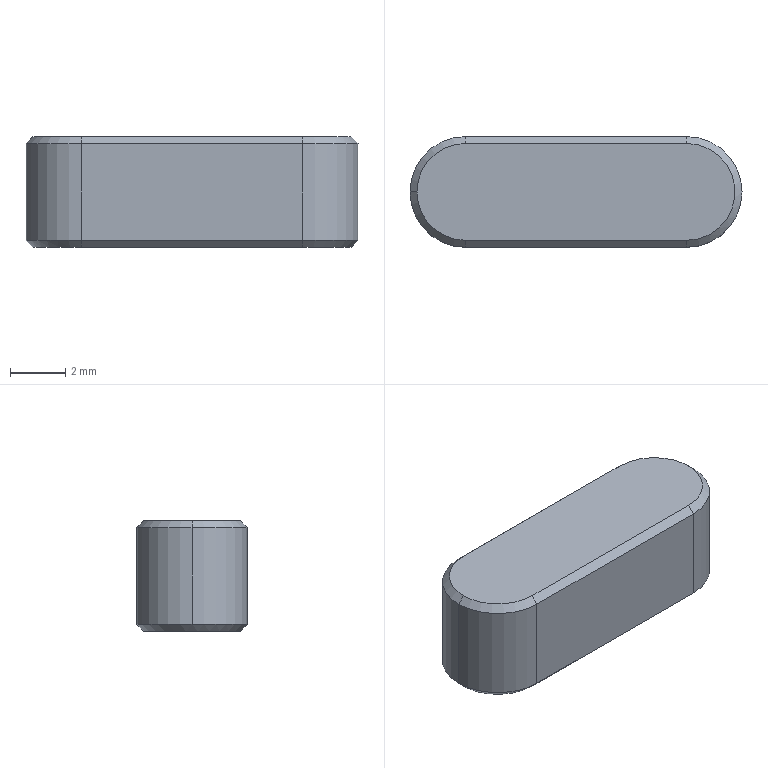Part | STEP file | Flat key Shanglong KEA-B4-L12-1 | 1 solid | 17 faces | box 12 x 4 x 4 mm | volume 176.513 mm3 | plane 8 | cone 6 | cylinder 3 | commonest cylinder face diameters 4 x3
STEP:
#1=CARTESIAN_POINT('',(4.,-1.75,0.000000414));
#2=VERTEX_POINT('',#1);
#3=CARTESIAN_POINT('',(5.75,0.,0.000000414));
#4=VERTEX_POINT('',#3);
#5=CARTESIAN_POINT('',(4.,0.,0.000000414));
#6=DIRECTION('',(0.,0.,1.));
#7=DIRECTION('',(1.,0.,0.));
#8=AXIS2_PLACEMENT_3D('',#5,#6,#7);
#9=CIRCLE('',#8,1.75);
#10=EDGE_CURVE('',#2,#4,#9,.T.);
#11=ORIENTED_EDGE('',*,*,#10,.T.);
#12=CARTESIAN_POINT('',(6.,0.,0.25));
#13=VERTEX_POINT('',#12);
#14=CARTESIAN_POINT('',(6.,0.,0.25));
#15=DIRECTION('',(0.7071,0.,0.7071));
#16=VECTOR('',#15,1000.);
#17=LINE('',#14,#16);
#18=EDGE_CURVE('',#4,#13,#17,.T.);
#19=ORIENTED_EDGE('',*,*,#18,.T.);
#20=CARTESIAN_POINT('',(4.,-2.,0.25));
#21=VERTEX_POINT('',#20);
#22=CARTESIAN_POINT('',(4.,0.,0.25));
#23=DIRECTION('',(0.,0.,-1.));
#24=DIRECTION('',(0.,-1.,0.));
#25=AXIS2_PLACEMENT_3D('',#22,#23,#24);
#26=CIRCLE('',#25,2.);
#27=EDGE_CURVE('',#13,#21,#26,.T.);
#28=ORIENTED_EDGE('',*,*,#27,.T.);
#29=CARTESIAN_POINT('',(4.,-2.,0.25));
#30=CARTESIAN_POINT('',(4.,-1.75,0.000000414));
#31=B_SPLINE_CURVE_WITH_KNOTS('',1,(#29,#30),.UNSPECIFIED.,.F.,.F.,(2,2),(0.,1.),.UNSPECIFIED.);
#32=EDGE_CURVE('',#21,#2,#31,.T.);
#33=ORIENTED_EDGE('',*,*,#32,.T.);
#34=EDGE_LOOP('',(#11,#19,#28,#33));
#35=FACE_OUTER_BOUND('',#34,.T.);
#36=CARTESIAN_POINT('',(4.,0.,0.25));
#37=DIRECTION('',(0.,0.,1.));
#38=DIRECTION('',(1.,0.,0.));
#39=AXIS2_PLACEMENT_3D('',#36,#37,#38);
#40=CONICAL_SURFACE('',#39,2.,0.7854);
#41=ADVANCED_FACE('',(#35),#40,.T.);
#42=CARTESIAN_POINT('',(-4.,-2.,3.75));
#43=VERTEX_POINT('',#42);
#44=CARTESIAN_POINT('',(-6.,0.,3.75));
#45=VERTEX_POINT('',#44);
#46=CARTESIAN_POINT('',(-4.,0.,3.75));
#47=DIRECTION('',(0.,0.,-1.));
#48=DIRECTION('',(-1.,0.,0.));
#49=AXIS2_PLACEMENT_3D('',#46,#47,#48);
#50=CIRCLE('',#49,2.);
#51=EDGE_CURVE('',#43,#45,#50,.T.);
#52=ORIENTED_EDGE('',*,*,#51,.T.);
#53=CARTESIAN_POINT('',(-6.,0.,0.25));
#54=VERTEX_POINT('',#53);
#55=CARTESIAN_POINT('',(-6.,0.,9.214));
#56=DIRECTION('',(0.,0.,-1.));
#57=VECTOR('',#56,1000.);
#58=LINE('',#55,#57);
#59=EDGE_CURVE('',#45,#54,#58,.T.);
#60=ORIENTED_EDGE('',*,*,#59,.T.);
#61=CARTESIAN_POINT('',(-4.,-2.,0.25));
#62=VERTEX_POINT('',#61);
#63=CARTESIAN_POINT('',(-4.,0.,0.25));
#64=DIRECTION('',(0.,0.,-1.));
#65=DIRECTION('',(0.,-1.,0.));
#66=AXIS2_PLACEMENT_3D('',#63,#64,#65);
#67=CIRCLE('',#66,2.);
#68=EDGE_CURVE('',#62,#54,#67,.T.);
#69=ORIENTED_EDGE('',*,*,#68,.F.);
#70=CARTESIAN_POINT('',(-4.,-2.,9.214));
#71=DIRECTION('',(0.,0.,1.));
#72=VECTOR('',#71,1000.);
#73=LINE('',#70,#72);
#74=EDGE_CURVE('',#62,#43,#73,.T.);
#75=ORIENTED_EDGE('',*,*,#74,.T.);
#76=EDGE_LOOP('',(#52,#60,#69,#75));
#77=FACE_OUTER_BOUND('',#76,.T.);
#78=CARTESIAN_POINT('',(-4.,0.,9.214));
#79=DIRECTION('',(0.,0.,-1.));
#80=DIRECTION('',(-1.,0.,0.));
#81=AXIS2_PLACEMENT_3D('',#78,#79,#80);
#82=CYLINDRICAL_SURFACE('',#81,2.);
#83=ADVANCED_FACE('',(#77),#82,.T.);
#84=CARTESIAN_POINT('',(-4.,-1.75,4.));
#85=VERTEX_POINT('',#84);
#86=CARTESIAN_POINT('',(-5.75,0.,4.));
#87=VERTEX_POINT('',#86);
#88=CARTESIAN_POINT('',(-4.,0.,4.));
#89=DIRECTION('',(0.,0.,-1.));
#90=DIRECTION('',(-1.,0.,0.));
#91=AXIS2_PLACEMENT_3D('',#88,#89,#90);
#92=CIRCLE('',#91,1.75);
#93=EDGE_CURVE('',#85,#87,#92,.T.);
#94=ORIENTED_EDGE('',*,*,#93,.T.);
#95=CARTESIAN_POINT('',(-6.,0.,3.75));
#96=DIRECTION('',(-0.7071,0.,-0.7071));
#97=VECTOR('',#96,1000.);
#98=LINE('',#95,#97);
#99=EDGE_CURVE('',#87,#45,#98,.T.);
#100=ORIENTED_EDGE('',*,*,#99,.T.);
#101=ORIENTED_EDGE('',*,*,#51,.F.);
#102=CARTESIAN_POINT('',(-4.,-499000.,-498994.486));
#103=DIRECTION('',(0.,0.7071,0.7071));
#104=VECTOR('',#103,1000.);
#105=LINE('',#102,#104);
#106=EDGE_CURVE('',#43,#85,#105,.T.);
#107=ORIENTED_EDGE('',*,*,#106,.T.);
#108=EDGE_LOOP('',(#94,#100,#101,#107));
#109=FACE_OUTER_BOUND('',#108,.T.);
#110=CARTESIAN_POINT('',(-4.,0.,3.75));
#111=DIRECTION('',(0.,0.,-1.));
#112=DIRECTION('',(-1.,0.,0.));
#113=AXIS2_PLACEMENT_3D('',#110,#111,#112);
#114=CONICAL_SURFACE('',#113,2.,0.7854);
#115=ADVANCED_FACE('',(#109),#114,.T.);
#116=CARTESIAN_POINT('',(4.,1.75,0.00000019));
#117=VERTEX_POINT('',#116);
#118=CARTESIAN_POINT('',(-4.,1.75,0.000000116));
#119=VERTEX_POINT('',#118);
#120=CARTESIAN_POINT('',(0.,1.75,0.));
#121=DIRECTION('',(-1.,0.,0.));
#122=VECTOR('',#121,1000.);
#123=LINE('',#120,#122);
#124=EDGE_CURVE('',#117,#119,#123,.T.);
#125=ORIENTED_EDGE('',*,*,#124,.F.);
#126=CARTESIAN_POINT('',(4.,0.,0.000000414));
#127=DIRECTION('',(0.,0.,1.));
#128=DIRECTION('',(1.,0.,0.));
#129=AXIS2_PLACEMENT_3D('',#126,#127,#128);
#130=CIRCLE('',#129,1.75);
#131=EDGE_CURVE('',#4,#117,#130,.T.);
#132=ORIENTED_EDGE('',*,*,#131,.F.);
#133=ORIENTED_EDGE('',*,*,#10,.F.);
#134=CARTESIAN_POINT('',(-4.,-1.75,0.000000207));
#135=VERTEX_POINT('',#134);
#136=CARTESIAN_POINT('',(0.,-1.75,0.));
#137=DIRECTION('',(1.,0.,0.));
#138=VECTOR('',#137,1000.);
#139=LINE('',#136,#138);
#140=EDGE_CURVE('',#135,#2,#139,.T.);
#141=ORIENTED_EDGE('',*,*,#140,.F.);
#142=CARTESIAN_POINT('',(-4.,0.,0.000000116));
#143=DIRECTION('',(0.,0.,1.));
#144=DIRECTION('',(1.,0.,0.));
#145=AXIS2_PLACEMENT_3D('',#142,#143,#144);
#146=CIRCLE('',#145,1.75);
#147=EDGE_CURVE('',#119,#135,#146,.T.);
#148=ORIENTED_EDGE('',*,*,#147,.F.);
#149=EDGE_LOOP('',(#125,#132,#133,#141,#148));
#150=FACE_OUTER_BOUND('',#149,.T.);
#151=CARTESIAN_POINT('',(0.,0.,0.));
#152=DIRECTION('',(0.,0.,1.));
#153=DIRECTION('',(1.,0.,0.));
#154=AXIS2_PLACEMENT_3D('',#151,#152,#153);
#155=PLANE('',#154);
#156=ADVANCED_FACE('',(#150),#155,.F.);
#157=CARTESIAN_POINT('',(-4.,2.,0.25));
#158=VERTEX_POINT('',#157);
#159=CARTESIAN_POINT('',(-4.,499000.,498998.486));
#160=DIRECTION('',(0.,-0.7071,-0.7071));
#161=VECTOR('',#160,1000.);
#162=LINE('',#159,#161);
#163=EDGE_CURVE('',#158,#119,#162,.T.);
#164=ORIENTED_EDGE('',*,*,#163,.T.);
#165=ORIENTED_EDGE('',*,*,#147,.T.);
#166=CARTESIAN_POINT('',(-4.,-1.75,0.000000207));
#167=CARTESIAN_POINT('',(-4.,-2.,0.25));
#168=B_SPLINE_CURVE_WITH_KNOTS('',1,(#166,#167),.UNSPECIFIED.,.F.,.F.,(2,2),(-0.000000138,1.),.UNSPECIFIED.);
#169=EDGE_CURVE('',#135,#62,#168,.T.);
#170=ORIENTED_EDGE('',*,*,#169,.T.);
#171=ORIENTED_EDGE('',*,*,#68,.T.);
#172=CARTESIAN_POINT('',(-4.,0.,0.25));
#173=DIRECTION('',(0.,0.,-1.));
#174=DIRECTION('',(0.,-1.,0.));
#175=AXIS2_PLACEMENT_3D('',#172,#173,#174);
#176=CIRCLE('',#175,2.);
#177=EDGE_CURVE('',#54,#158,#176,.T.);
#178=ORIENTED_EDGE('',*,*,#177,.T.);
#179=EDGE_LOOP('',(#164,#165,#170,#171,#178));
#180=FACE_OUTER_BOUND('',#179,.T.);
#181=CARTESIAN_POINT('',(-4.,0.,0.25));
#182=DIRECTION('',(0.,0.,1.));
#183=DIRECTION('',(1.,0.,0.));
#184=AXIS2_PLACEMENT_3D('',#181,#182,#183);
#185=CONICAL_SURFACE('',#184,2.,0.7854);
#186=ADVANCED_FACE('',(#180),#185,.T.);
#187=CARTESIAN_POINT('',(4.,2.,0.25));
#188=VERTEX_POINT('',#187);
#189=CARTESIAN_POINT('',(4.,1.875,0.125));
#190=DIRECTION('',(0.,-0.7071,-0.7071));
#191=VECTOR('',#190,1000.);
#192=LINE('',#189,#191);
#193=EDGE_CURVE('',#188,#117,#192,.T.);
#194=ORIENTED_EDGE('',*,*,#193,.T.);
#195=ORIENTED_EDGE('',*,*,#124,.T.);
#196=ORIENTED_EDGE('',*,*,#163,.F.);
#197=CARTESIAN_POINT('',(0.,2.,0.25));
#198=DIRECTION('',(1.,0.,0.));
#199=VECTOR('',#198,1000.);
#200=LINE('',#197,#199);
#201=EDGE_CURVE('',#158,#188,#200,.T.);
#202=ORIENTED_EDGE('',*,*,#201,.T.);
#203=EDGE_LOOP('',(#194,#195,#196,#202));
#204=FACE_OUTER_BOUND('',#203,.T.);
#205=CARTESIAN_POINT('',(0.,1.875,0.125));
#206=DIRECTION('',(0.,0.7071,-0.7071));
#207=DIRECTION('',(0.,0.7071,0.7071));
#208=AXIS2_PLACEMENT_3D('',#205,#206,#207);
#209=PLANE('',#208);
#210=ADVANCED_FACE('',(#204),#209,.T.);
#211=ORIENTED_EDGE('',*,*,#18,.F.);
#212=ORIENTED_EDGE('',*,*,#131,.T.);
#213=ORIENTED_EDGE('',*,*,#193,.F.);
#214=CARTESIAN_POINT('',(4.,0.,0.25));
#215=DIRECTION('',(0.,0.,-1.));
#216=DIRECTION('',(0.,-1.,0.));
#217=AXIS2_PLACEMENT_3D('',#214,#215,#216);
#218=CIRCLE('',#217,2.);
#219=EDGE_CURVE('',#188,#13,#218,.T.);
#220=ORIENTED_EDGE('',*,*,#219,.T.);
#221=EDGE_LOOP('',(#211,#212,#213,#220));
#222=FACE_OUTER_BOUND('',#221,.T.);
#223=CARTESIAN_POINT('',(4.,0.,0.25));
#224=DIRECTION('',(0.,0.,1.));
#225=DIRECTION('',(1.,0.,0.));
#226=AXIS2_PLACEMENT_3D('',#223,#224,#225);
#227=CONICAL_SURFACE('',#226,2.,0.7854);
#228=ADVANCED_FACE('',(#222),#227,.T.);
#229=ORIENTED_EDGE('',*,*,#169,.F.);
#230=ORIENTED_EDGE('',*,*,#140,.T.);
#231=ORIENTED_EDGE('',*,*,#32,.F.);
#232=CARTESIAN_POINT('',(0.,-2.,0.25));
#233=DIRECTION('',(-1.,0.,0.));
#234=VECTOR('',#233,1000.);
#235=LINE('',#232,#234);
#236=EDGE_CURVE('',#21,#62,#235,.T.);
#237=ORIENTED_EDGE('',*,*,#236,.T.);
#238=EDGE_LOOP('',(#229,#230,#231,#237));
#239=FACE_OUTER_BOUND('',#238,.T.);
#240=CARTESIAN_POINT('',(0.,-1.875,0.125));
#241=DIRECTION('',(0.,-0.7071,-0.7071));
#242=DIRECTION('',(0.,0.7071,-0.7071));
#243=AXIS2_PLACEMENT_3D('',#240,#241,#242);
#244=PLANE('',#243);
#245=ADVANCED_FACE('',(#239),#244,.T.);
#246=ORIENTED_EDGE('',*,*,#59,.F.);
#247=CARTESIAN_POINT('',(-4.,2.,3.75));
#248=VERTEX_POINT('',#247);
#249=CARTESIAN_POINT('',(-4.,0.,3.75));
#250=DIRECTION('',(0.,0.,-1.));
#251=DIRECTION('',(-1.,0.,0.));
#252=AXIS2_PLACEMENT_3D('',#249,#250,#251);
#253=CIRCLE('',#252,2.);
#254=EDGE_CURVE('',#45,#248,#253,.T.);
#255=ORIENTED_EDGE('',*,*,#254,.T.);
#256=CARTESIAN_POINT('',(-4.,2.,9.214));
#257=DIRECTION('',(0.,0.,-1.));
#258=VECTOR('',#257,1000.);
#259=LINE('',#256,#258);
#260=EDGE_CURVE('',#248,#158,#259,.T.);
#261=ORIENTED_EDGE('',*,*,#260,.T.);
#262=ORIENTED_EDGE('',*,*,#177,.F.);
#263=EDGE_LOOP('',(#246,#255,#261,#262));
#264=FACE_OUTER_BOUND('',#263,.T.);
#265=CARTESIAN_POINT('',(-4.,0.,9.214));
#266=DIRECTION('',(0.,0.,-1.));
#267=DIRECTION('',(-1.,0.,0.));
#268=AXIS2_PLACEMENT_3D('',#265,#266,#267);
#269=CYLINDRICAL_SURFACE('',#268,2.);
#270=ADVANCED_FACE('',(#264),#269,.T.);
#271=ORIENTED_EDGE('',*,*,#260,.F.);
#272=CARTESIAN_POINT('',(4.,2.,3.75));
#273=VERTEX_POINT('',#272);
#274=CARTESIAN_POINT('',(6.,2.,3.75));
#275=DIRECTION('',(1.,0.,0.));
#276=VECTOR('',#275,1000.);
#277=LINE('',#274,#276);
#278=EDGE_CURVE('',#248,#273,#277,.T.);
#279=ORIENTED_EDGE('',*,*,#278,.T.);
#280=CARTESIAN_POINT('',(4.,2.,0.));
#281=DIRECTION('',(0.,0.,-1.));
#282=VECTOR('',#281,1000.);
#283=LINE('',#280,#282);
#284=EDGE_CURVE('',#273,#188,#283,.T.);
#285=ORIENTED_EDGE('',*,*,#284,.T.);
#286=ORIENTED_EDGE('',*,*,#201,.F.);
#287=EDGE_LOOP('',(#271,#279,#285,#286));
#288=FACE_OUTER_BOUND('',#287,.T.);
#289=CARTESIAN_POINT('',(6.,2.,0.));
#290=DIRECTION('',(0.,1.,0.));
#291=DIRECTION('',(0.,0.,1.));
#292=AXIS2_PLACEMENT_3D('',#289,#290,#291);
#293=PLANE('',#292);
#294=ADVANCED_FACE('',(#288),#293,.T.);
#295=ORIENTED_EDGE('',*,*,#284,.F.);
#296=CARTESIAN_POINT('',(4.,-2.,3.75));
#297=VERTEX_POINT('',#296);
#298=CARTESIAN_POINT('',(4.,0.,3.75));
#299=DIRECTION('',(0.,0.,-1.));
#300=DIRECTION('',(-1.,0.,0.));
#301=AXIS2_PLACEMENT_3D('',#298,#299,#300);
#302=CIRCLE('',#301,2.);
#303=EDGE_CURVE('',#273,#297,#302,.T.);
#304=ORIENTED_EDGE('',*,*,#303,.T.);
#305=CARTESIAN_POINT('',(4.,-2.,9.214));
#306=DIRECTION('',(0.,0.,-1.));
#307=VECTOR('',#306,1000.);
#308=LINE('',#305,#307);
#309=EDGE_CURVE('',#297,#21,#308,.T.);
#310=ORIENTED_EDGE('',*,*,#309,.T.);
#311=ORIENTED_EDGE('',*,*,#27,.F.);
#312=ORIENTED_EDGE('',*,*,#219,.F.);
#313=EDGE_LOOP('',(#295,#304,#310,#311,#312));
#314=FACE_OUTER_BOUND('',#313,.T.);
#315=CARTESIAN_POINT('',(4.,0.,9.214));
#316=DIRECTION('',(0.,0.,-1.));
#317=DIRECTION('',(-1.,0.,0.));
#318=AXIS2_PLACEMENT_3D('',#315,#316,#317);
#319=CYLINDRICAL_SURFACE('',#318,2.);
#320=ADVANCED_FACE('',(#314),#319,.T.);
#321=ORIENTED_EDGE('',*,*,#309,.F.);
#322=CARTESIAN_POINT('',(-6.,-2.,3.75));
#323=DIRECTION('',(-1.,0.,0.));
#324=VECTOR('',#323,1000.);
#325=LINE('',#322,#324);
#326=EDGE_CURVE('',#297,#43,#325,.T.);
#327=ORIENTED_EDGE('',*,*,#326,.T.);
#328=ORIENTED_EDGE('',*,*,#74,.F.);
#329=ORIENTED_EDGE('',*,*,#236,.F.);
#330=EDGE_LOOP('',(#321,#327,#328,#329));
#331=FACE_OUTER_BOUND('',#330,.T.);
#332=CARTESIAN_POINT('',(-6.,-2.,0.));
#333=DIRECTION('',(0.,-1.,0.));
#334=DIRECTION('',(0.,0.,-1.));
#335=AXIS2_PLACEMENT_3D('',#332,#333,#334);
#336=PLANE('',#335);
#337=ADVANCED_FACE('',(#331),#336,.T.);
#338=ORIENTED_EDGE('',*,*,#99,.F.);
#339=CARTESIAN_POINT('',(-4.,1.75,4.));
#340=VERTEX_POINT('',#339);
#341=CARTESIAN_POINT('',(-4.,0.,4.));
#342=DIRECTION('',(0.,0.,-1.));
#343=DIRECTION('',(-1.,0.,0.));
#344=AXIS2_PLACEMENT_3D('',#341,#342,#343);
#345=CIRCLE('',#344,1.75);
#346=EDGE_CURVE('',#87,#340,#345,.T.);
#347=ORIENTED_EDGE('',*,*,#346,.T.);
#348=CARTESIAN_POINT('',(-4.,1.75,4.));
#349=CARTESIAN_POINT('',(-4.,2.,3.75));
#350=B_SPLINE_CURVE_WITH_KNOTS('',1,(#348,#349),.UNSPECIFIED.,.F.,.F.,(2,2),(-0.000000597,1.),.UNSPECIFIED.);
#351=EDGE_CURVE('',#340,#248,#350,.T.);
#352=ORIENTED_EDGE('',*,*,#351,.T.);
#353=ORIENTED_EDGE('',*,*,#254,.F.);
#354=EDGE_LOOP('',(#338,#347,#352,#353));
#355=FACE_OUTER_BOUND('',#354,.T.);
#356=CARTESIAN_POINT('',(-4.,0.,3.75));
#357=DIRECTION('',(0.,0.,-1.));
#358=DIRECTION('',(-1.,0.,0.));
#359=AXIS2_PLACEMENT_3D('',#356,#357,#358);
#360=CONICAL_SURFACE('',#359,2.,0.7854);
#361=ADVANCED_FACE('',(#355),#360,.T.);
#362=ORIENTED_EDGE('',*,*,#351,.F.);
#363=CARTESIAN_POINT('',(4.,1.75,4.));
#364=VERTEX_POINT('',#363);
#365=CARTESIAN_POINT('',(0.,1.75,4.));
#366=DIRECTION('',(1.,0.,0.));
#367=VECTOR('',#366,1000.);
#368=LINE('',#365,#367);
#369=EDGE_CURVE('',#340,#364,#368,.T.);
#370=ORIENTED_EDGE('',*,*,#369,.T.);
#371=CARTESIAN_POINT('',(4.,1.875,3.875));
#372=DIRECTION('',(0.,0.7071,-0.7071));
#373=VECTOR('',#372,1000.);
#374=LINE('',#371,#373);
#375=EDGE_CURVE('',#364,#273,#374,.T.);
#376=ORIENTED_EDGE('',*,*,#375,.T.);
#377=ORIENTED_EDGE('',*,*,#278,.F.);
#378=EDGE_LOOP('',(#362,#370,#376,#377));
#379=FACE_OUTER_BOUND('',#378,.T.);
#380=CARTESIAN_POINT('',(0.,1.875,3.875));
#381=DIRECTION('',(0.,0.7071,0.7071));
#382=DIRECTION('',(0.,-0.7071,0.7071));
#383=AXIS2_PLACEMENT_3D('',#380,#381,#382);
#384=PLANE('',#383);
#385=ADVANCED_FACE('',(#379),#384,.T.);
#386=ORIENTED_EDGE('',*,*,#375,.F.);
#387=CARTESIAN_POINT('',(4.,-1.75,4.));
#388=VERTEX_POINT('',#387);
#389=CARTESIAN_POINT('',(4.,0.,4.));
#390=DIRECTION('',(0.,0.,-1.));
#391=DIRECTION('',(-1.,0.,0.));
#392=AXIS2_PLACEMENT_3D('',#389,#390,#391);
#393=CIRCLE('',#392,1.75);
#394=EDGE_CURVE('',#364,#388,#393,.T.);
#395=ORIENTED_EDGE('',*,*,#394,.T.);
#396=CARTESIAN_POINT('',(4.,-1.75,4.));
#397=CARTESIAN_POINT('',(4.,-2.,3.75));
#398=B_SPLINE_CURVE_WITH_KNOTS('',1,(#396,#397),.UNSPECIFIED.,.F.,.F.,(2,2),(0.,1.),.UNSPECIFIED.);
#399=EDGE_CURVE('',#388,#297,#398,.T.);
#400=ORIENTED_EDGE('',*,*,#399,.T.);
#401=ORIENTED_EDGE('',*,*,#303,.F.);
#402=EDGE_LOOP('',(#386,#395,#400,#401));
#403=FACE_OUTER_BOUND('',#402,.T.);
#404=CARTESIAN_POINT('',(4.,0.,3.75));
#405=DIRECTION('',(0.,0.,-1.));
#406=DIRECTION('',(-1.,0.,0.));
#407=AXIS2_PLACEMENT_3D('',#404,#405,#406);
#408=CONICAL_SURFACE('',#407,2.,0.7854);
#409=ADVANCED_FACE('',(#403),#408,.T.);
#410=ORIENTED_EDGE('',*,*,#399,.F.);
#411=CARTESIAN_POINT('',(0.,-1.75,4.));
#412=DIRECTION('',(-1.,0.,0.));
#413=VECTOR('',#412,1000.);
#414=LINE('',#411,#413);
#415=EDGE_CURVE('',#388,#85,#414,.T.);
#416=ORIENTED_EDGE('',*,*,#415,.T.);
#417=ORIENTED_EDGE('',*,*,#106,.F.);
#418=ORIENTED_EDGE('',*,*,#326,.F.);
#419=EDGE_LOOP('',(#410,#416,#417,#418));
#420=FACE_OUTER_BOUND('',#419,.T.);
#421=CARTESIAN_POINT('',(0.,-1.875,3.875));
#422=DIRECTION('',(0.,-0.7071,0.7071));
#423=DIRECTION('',(0.,-0.7071,-0.7071));
#424=AXIS2_PLACEMENT_3D('',#421,#422,#423);
#425=PLANE('',#424);
#426=ADVANCED_FACE('',(#420),#425,.T.);
#427=ORIENTED_EDGE('',*,*,#394,.F.);
#428=ORIENTED_EDGE('',*,*,#369,.F.);
#429=ORIENTED_EDGE('',*,*,#346,.F.);
#430=ORIENTED_EDGE('',*,*,#93,.F.);
#431=ORIENTED_EDGE('',*,*,#415,.F.);
#432=EDGE_LOOP('',(#427,#428,#429,#430,#431));
#433=FACE_OUTER_BOUND('',#432,.T.);
#434=CARTESIAN_POINT('',(0.,0.,4.));
#435=DIRECTION('',(0.,0.,1.));
#436=DIRECTION('',(1.,0.,0.));
#437=AXIS2_PLACEMENT_3D('',#434,#435,#436);
#438=PLANE('',#437);
#439=ADVANCED_FACE('',(#433),#438,.T.);
#440=CLOSED_SHELL('',(#41,#83,#115,#156,#186,#210,#228,#245,#270,#294,#320,#337,#361,#385,#409,#426,#439));
#441=MANIFOLD_SOLID_BREP('',#440);
#442=CARTESIAN_POINT('',(0.,0.,0.));
#443=DIRECTION('',(0.,0.,1.));
#444=DIRECTION('',(1.,0.,0.));
#445=AXIS2_PLACEMENT_3D('',#442,#443,#444);
#446=(LENGTH_UNIT()NAMED_UNIT(*)SI_UNIT(.MILLI.,.METRE.));
#447=UNCERTAINTY_MEASURE_WITH_UNIT(LENGTH_MEASURE(0.00001),#446,'','');
#448=(NAMED_UNIT(*)PLANE_ANGLE_UNIT()SI_UNIT($,.RADIAN.));
#449=(NAMED_UNIT(*)SI_UNIT($,.STERADIAN.)SOLID_ANGLE_UNIT());
#450=(GEOMETRIC_REPRESENTATION_CONTEXT(3)GLOBAL_UNCERTAINTY_ASSIGNED_CONTEXT((#447))GLOBAL_UNIT_ASSIGNED_CONTEXT((#446,#448,#449))REPRESENTATION_CONTEXT('',''));
#451=ADVANCED_BREP_SHAPE_REPRESENTATION('',(#441,#445),#450);